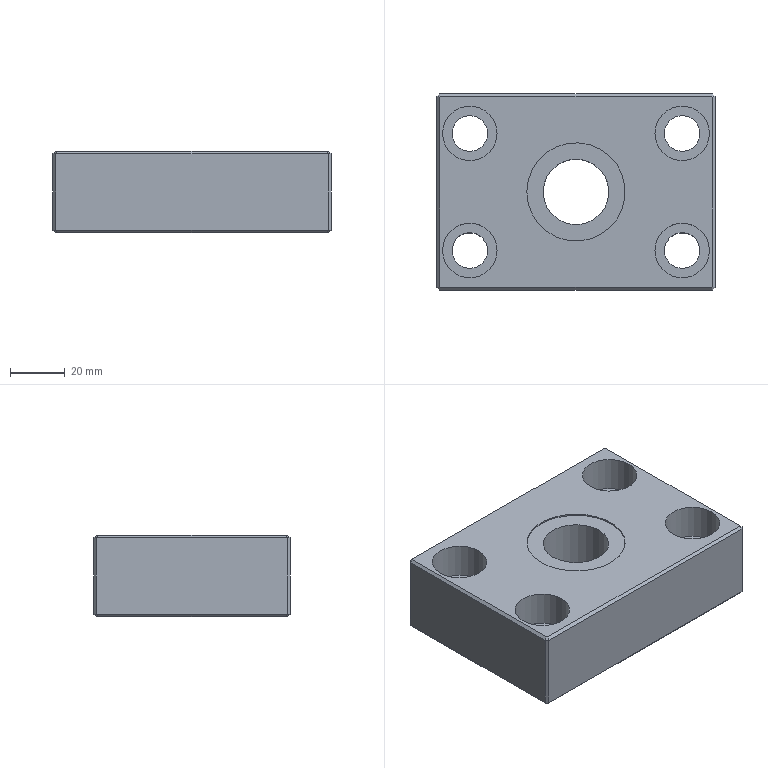CAM job | NX | 3-axis milling, drilling | part box 102 x 72 x 30 mm | stock box 106 x 75 x 35 mm
Tools:
number,name,description,diameter,corner_radius,flute_length,length,flutes
9,D3-9-D4-50-3T-ROUGH,D3-9-D4-50-3T,3.0,0.0,9.0,10.0,3
10,D3-9-D4-50-3T-FINISH,D3-9-D4-50-3T-精,3.0,0.0,9.0,10.0,2
2,D12-36-D12-75-3T-ROUGH,D12-36-D12-75-3T,12.0,0.0,36.0,75.0,3
3,D12-36-D12-120-3T-FINISH,D12-55-D12-120-3T,12.0,0.0,55.0,120.0,3
1,D80-FACE-MILL,D80面刀,80.0,0.0,30.0,30.0,5
5,CHAMFER-D6-90DEG,倒角D6-90度,6.0,0.0,5.0,50.0,2
4,CHAMFER-D10-90DEG,倒角D10-90度,10.0,0.0,10.0,75.0,2
6,D13DRILL ,Drilling Tool,13.0,0.0,35.0,50.0,2
7,D20PLUNGE-MILL,Milling Tool-5 Parameters,20.0,0.0,30.0,30.0,4
0,G3-4,Thread Mill,15.7,0.0,50.0,50.0,2
Operations:
program,operation,operation_type,tool,method,geometry_group,spindle_rpm,surface_speed,feed_per_tooth,feed_cut,feed_plunge,cut_length_mm,path_length_mm,cut_time_min,machine_time_min
A1,PLANAR_MILL,PlanarMilling,D80-FACE-MILL,METHOD,A-G54,3500.0,879.0,0.0457,800.0,100.0,196.0,231.94,0.245,0.2486
A1,ADAPTIVE_MILLING,CavityMilling,D12-36-D12-75-3T-ROUGH,METHOD,WORKPIECE_54,4500.0,169.0,0.2222,3000.0,100.0,2928.762,3158.244,0.9763,0.9992
A1,PLANAR_MILL_2,PlanarMilling,D12-36-D12-75-3T-ROUGH,METHOD,WORKPIECE_54,4500.0,169.0,0.0741,1000.0,100.0,155.988,194.388,0.156,0.1598
A1,PLANAR_MILL_2_COPY_COPY_COPY,PlanarMilling,D12-36-D12-75-3T-ROUGH,METHOD,WORKPIECE_54,4000.0,150.0,0.0667,800.0,100.0,50.553,127.553,0.0632,0.0709
A1,PLANAR_MILL_1,PlanarMilling,D12-36-D12-120-3T-FINISH,METHOD,WORKPIECE_54,4000.0,150.0,0.0667,800.0,100.0,786.453,987.638,0.9831,1.003
A1,PLANAR_MILL_2_COPY,PlanarMilling,D12-36-D12-120-3T-FINISH,METHOD,WORKPIECE_54,4400.0,165.0,0.0227,300.0,100.0,96.516,133.516,0.3217,0.3254
A1,PLANAR_MILL_2_COPY_COPY,PlanarMilling,D12-36-D12-120-3T-FINISH,METHOD,WORKPIECE_54,4000.0,150.0,0.0667,800.0,100.0,49.054,146.054,0.0613,0.071
A1,DRILLING,Operation,CHAMFER-D10-90DEG,METHOD,WORKPIECE_54,2000.0,62.0,0.05,200.0,0.0,18.0,248.867,0.09,0.1131
A1,DRILLING_COPY,Operation,D13DRILL ,METHOD,WORKPIECE_54,1600.0,65.0,0.0625,200.0,0.0,152.0,516.867,0.76,0.7965
A1,DRILLING_COPY_COPY,Operation,D20PLUNGE-MILL,METHOD,WORKPIECE_54,1200.0,75.0,0.0125,60.0,0.0,64.0,340.867,1.067,1.094
A1,PLANAR_MILL_3,PlanarMilling,CHAMFER-D6-90DEG,METHOD,WORKPIECE_54,3000.0,56.0,0.1667,1000.0,100.0,257.284,576.986,0.2573,0.2893
A1,PLANAR_MILL_3_COPY_1,PlanarMilling,CHAMFER-D6-90DEG,METHOD,WORKPIECE_54,3000.0,56.0,0.1667,1000.0,100.0,175.161,598.864,0.1752,0.2175
A1,PLANAR_MILL_3_COPY,PlanarMilling,CHAMFER-D6-90DEG,METHOD,WORKPIECE_54,3000.0,56.0,0.1667,1000.0,100.0,120.498,157.298,0.1205,0.1242
A1,PLANAR_MILL_3_COPY_COPY,PlanarMilling,CHAMFER-D6-90DEG,METHOD,WORKPIECE_54,3000.0,56.0,0.1,600.0,100.0,79.848,121.448,0.1331,0.1372
A1,PLANAR_MILL_4,PlanarMilling,CHAMFER-D6-90DEG,METHOD,WORKPIECE_54,3000.0,56.0,0.1667,1000.0,100.0,361.879,401.879,0.3619,0.3659
A1,THREAD_MILLING,ThreadMilling,G3-4,METHOD,WORKPIECE_54,4000.0,197.0,0.0375,300.0,100.0,263.029,347.403,0.8768,0.8852
A1,PLANAR_MILL_COPY,PlanarMilling,D80-FACE-MILL,METHOD,A-G54,4500.0,1130.0,0.0267,600.0,100.0,196.0,232.0,0.3267,0.3303
B1,PLANAR_MILL_COPY_1,PlanarMilling,D80-FACE-MILL,METHOD,B-G55,3500.0,879.0,0.0686,1200.0,100.0,980.0,2057.94,0.8167,0.9245
B1,PLANAR_MILL_5,PlanarMilling,D3-9-D4-50-3T-ROUGH,METHOD,B-G55,4500.0,42.0,0.0593,800.0,100.0,1576.469,1637.119,1.971,1.977
B1,PLANAR_MILL_5_COPY,PlanarMilling,D3-9-D4-50-3T-ROUGH,METHOD,B-G55,4500.0,42.0,0.0593,800.0,100.0,1584.637,1645.287,1.981,1.987
B1,PLANAR_MILL_5_COPY_1,PlanarMilling,D3-9-D4-50-3T-FINISH,METHOD,B-G55,4000.0,37.0,0.1,800.0,100.0,187.783,249.283,0.2347,0.2409
B1,PLANAR_MILL_5_COPY_COPY,PlanarMilling,D3-9-D4-50-3T-FINISH,METHOD,B-G55,4000.0,37.0,0.1,800.0,100.0,197.242,258.742,0.2466,0.2527
B1,PLANAR_MILL_6,PlanarMilling,CHAMFER-D6-90DEG,METHOD,B-G55,3500.0,65.0,0.1429,1000.0,100.0,238.368,703.223,0.2384,0.2849
B1,PLANAR_MILL_6_COPY,PlanarMilling,CHAMFER-D6-90DEG,METHOD,B-G55,3500.0,65.0,0.1429,1000.0,100.0,200.216,258.216,0.2002,0.206
B1,PLANAR_MILL_6_COPY_COPY,PlanarMilling,CHAMFER-D6-90DEG,METHOD,B-G55,3500.0,65.0,0.1429,1000.0,100.0,185.465,243.465,0.1855,0.1913
B1,PLANAR_MILL_6_COPY_COPY_COPY,PlanarMilling,CHAMFER-D6-90DEG,METHOD,B-G55,3500.0,65.0,0.1429,1000.0,100.0,362.806,423.406,0.3628,0.3689
B1,PLANAR_MILL_COPY_1_COPY,PlanarMilling,D80-FACE-MILL,METHOD,B-G55,3500.0,879.0,0.0457,800.0,100.0,196.0,262.0,0.245,0.2516